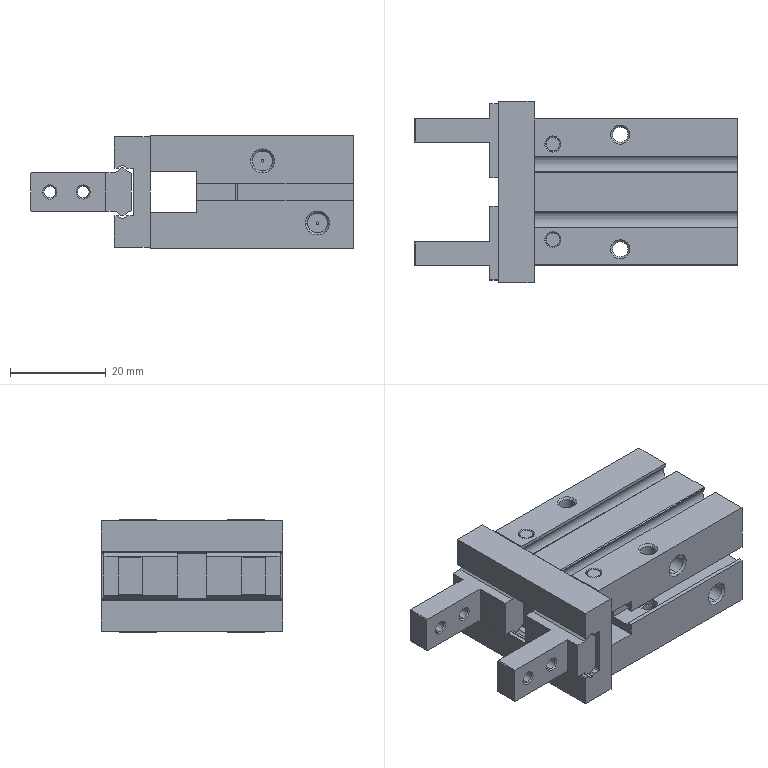Part | SolidWorks | features BaseBody 3, MoveCopyBody 2 | 3 solids | 249 faces | box 67.5 x 38 x 23.6 mm | volume 30087 mm3 | plane 116 | cylinder 71 | cone 62 | commonest cylinder face diameters 3.242 x16 0.4 x10 2.459 x8 1 x6 4.02 x6 4.2 x6